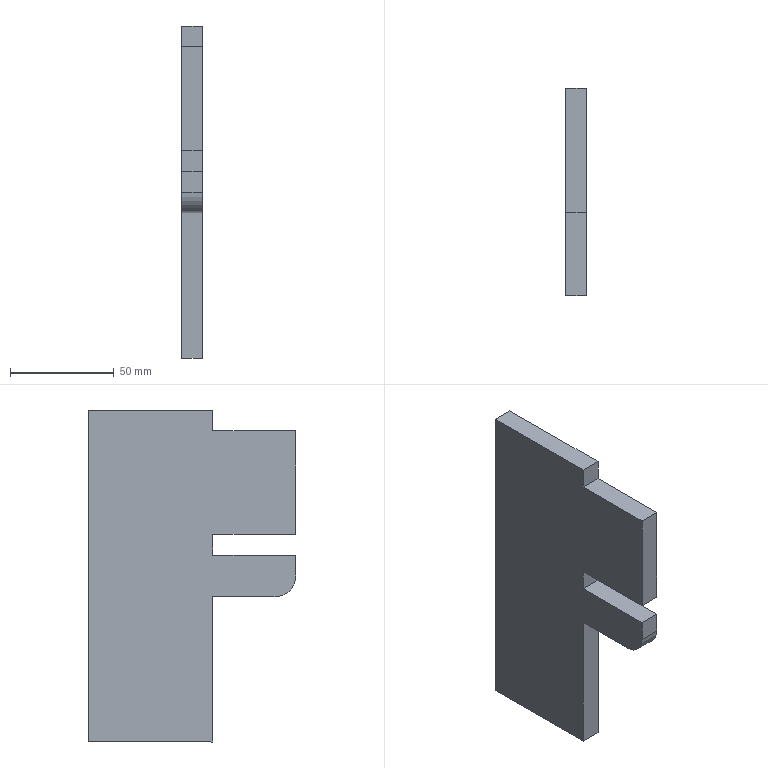Part | STEP file | cylinder mounting plate reinforcement--000.001--20240928 | 1 solid | 15 faces | box 10 x 100 x 160 mm | volume 123785 mm3 | plane 14 | cylinder 1 | commonest cylinder face diameters 20 x1
STEP:
#1=CARTESIAN_POINT('',(0.,0.,0.));
#2=DIRECTION('',(0.,0.,1.));
#3=DIRECTION('',(1.,0.,0.));
#4=AXIS2_PLACEMENT_3D('',#1,#2,#3);
#5=CARTESIAN_POINT('',(0.,-60.,90.));
#6=VERTEX_POINT('',#5);
#7=CARTESIAN_POINT('',(-10.,-60.,90.));
#8=VERTEX_POINT('',#7);
#9=CARTESIAN_POINT('',(657.,-60.,90.));
#10=DIRECTION('',(-1.,0.,0.));
#11=VECTOR('',#10,1.);
#12=LINE('',#9,#11);
#13=CARTESIAN_POINT('',(-221.5,-60.,-40.));
#14=DIRECTION('',(0.,-1.,0.));
#15=DIRECTION('',(-1.,0.,0.));
#16=AXIS2_PLACEMENT_3D('',#13,#14,#15);
#17=PLANE('',#16);
#18=CARTESIAN_POINT('',(-878.5,-130.));
#19=DIRECTION('',(1.,0.));
#20=VECTOR('',#19,1.);
#21=LINE('',#18,#20);
#22=(GEOMETRIC_REPRESENTATION_CONTEXT(2)PARAMETRIC_REPRESENTATION_CONTEXT()REPRESENTATION_CONTEXT('',''));
#23=DEFINITIONAL_REPRESENTATION('',(#21),#22);
#24=PCURVE('',#17,#23);
#25=CARTESIAN_POINT('',(657.,0.,90.));
#26=DIRECTION('',(0.,0.,1.));
#27=DIRECTION('',(0.,1.,0.));
#28=AXIS2_PLACEMENT_3D('',#25,#26,#27);
#29=PLANE('',#28);
#30=CARTESIAN_POINT('',(-60.,0.));
#31=DIRECTION('',(0.,1.));
#32=VECTOR('',#31,1.);
#33=LINE('',#30,#32);
#34=(GEOMETRIC_REPRESENTATION_CONTEXT(2)PARAMETRIC_REPRESENTATION_CONTEXT()REPRESENTATION_CONTEXT('',''));
#35=DEFINITIONAL_REPRESENTATION('',(#33),#34);
#36=PCURVE('',#29,#35);
#37=SURFACE_CURVE('',#12,(#24,#36),.PCURVE_S1.);
#38=EDGE_CURVE('',#6,#8,#37,.T.);
#39=ORIENTED_EDGE('',*,*,#38,.F.);
#40=CARTESIAN_POINT('',(0.,-60.,100.));
#41=VERTEX_POINT('',#40);
#42=CARTESIAN_POINT('',(0.,-60.,-40.));
#43=DIRECTION('',(0.,0.,1.));
#44=VECTOR('',#43,1.);
#45=LINE('',#42,#44);
#46=CARTESIAN_POINT('',(-221.5,0.));
#47=DIRECTION('',(0.,-1.));
#48=VECTOR('',#47,1.);
#49=LINE('',#46,#48);
#50=(GEOMETRIC_REPRESENTATION_CONTEXT(2)PARAMETRIC_REPRESENTATION_CONTEXT()REPRESENTATION_CONTEXT('',''));
#51=DEFINITIONAL_REPRESENTATION('',(#49),#50);
#52=PCURVE('',#17,#51);
#53=CARTESIAN_POINT('',(0.,-60.,1330.173));
#54=DIRECTION('',(-1.,0.,0.));
#55=DIRECTION('',(0.,-0.2756,-0.9613));
#56=AXIS2_PLACEMENT_3D('',#53,#54,#55);
#57=PLANE('',#56);
#58=CARTESIAN_POINT('',(1317.095,-377.671));
#59=DIRECTION('',(-0.9613,0.2756));
#60=VECTOR('',#59,1.);
#61=LINE('',#58,#60);
#62=(GEOMETRIC_REPRESENTATION_CONTEXT(2)PARAMETRIC_REPRESENTATION_CONTEXT()REPRESENTATION_CONTEXT('',''));
#63=DEFINITIONAL_REPRESENTATION('',(#61),#62);
#64=PCURVE('',#57,#63);
#65=SURFACE_CURVE('',#45,(#52,#64),.PCURVE_S1.);
#66=EDGE_CURVE('',#6,#41,#65,.T.);
#67=ORIENTED_EDGE('',*,*,#66,.T.);
#68=CARTESIAN_POINT('',(-10.,-60.,100.));
#69=VERTEX_POINT('',#68);
#70=CARTESIAN_POINT('',(657.,-60.,100.));
#71=DIRECTION('',(-1.,0.,0.));
#72=VECTOR('',#71,1.);
#73=LINE('',#70,#72);
#74=CARTESIAN_POINT('',(-878.5,-140.));
#75=DIRECTION('',(1.,0.));
#76=VECTOR('',#75,1.);
#77=LINE('',#74,#76);
#78=(GEOMETRIC_REPRESENTATION_CONTEXT(2)PARAMETRIC_REPRESENTATION_CONTEXT()REPRESENTATION_CONTEXT('',''));
#79=DEFINITIONAL_REPRESENTATION('',(#77),#78);
#80=PCURVE('',#17,#79);
#81=CARTESIAN_POINT('',(657.,0.,100.));
#82=DIRECTION('',(0.,0.,1.));
#83=DIRECTION('',(0.,1.,0.));
#84=AXIS2_PLACEMENT_3D('',#81,#82,#83);
#85=PLANE('',#84);
#86=CARTESIAN_POINT('',(-60.,0.));
#87=DIRECTION('',(0.,1.));
#88=VECTOR('',#87,1.);
#89=LINE('',#86,#88);
#90=(GEOMETRIC_REPRESENTATION_CONTEXT(2)PARAMETRIC_REPRESENTATION_CONTEXT()REPRESENTATION_CONTEXT('',''));
#91=DEFINITIONAL_REPRESENTATION('',(#89),#90);
#92=PCURVE('',#85,#91);
#93=SURFACE_CURVE('',#73,(#80,#92),.PCURVE_S1.);
#94=EDGE_CURVE('',#41,#69,#93,.T.);
#95=ORIENTED_EDGE('',*,*,#94,.T.);
#96=CARTESIAN_POINT('',(-10.,-60.,-40.));
#97=DIRECTION('',(0.,0.,1.));
#98=VECTOR('',#97,1.);
#99=LINE('',#96,#98);
#100=CARTESIAN_POINT('',(-211.5,0.));
#101=DIRECTION('',(0.,-1.));
#102=VECTOR('',#101,1.);
#103=LINE('',#100,#102);
#104=(GEOMETRIC_REPRESENTATION_CONTEXT(2)PARAMETRIC_REPRESENTATION_CONTEXT()REPRESENTATION_CONTEXT('',''));
#105=DEFINITIONAL_REPRESENTATION('',(#103),#104);
#106=PCURVE('',#17,#105);
#107=CARTESIAN_POINT('',(-10.,-60.,1330.173));
#108=DIRECTION('',(-1.,0.,0.));
#109=DIRECTION('',(0.,-0.2756,-0.9613));
#110=AXIS2_PLACEMENT_3D('',#107,#108,#109);
#111=PLANE('',#110);
#112=CARTESIAN_POINT('',(1317.095,-377.671));
#113=DIRECTION('',(-0.9613,0.2756));
#114=VECTOR('',#113,1.);
#115=LINE('',#112,#114);
#116=(GEOMETRIC_REPRESENTATION_CONTEXT(2)PARAMETRIC_REPRESENTATION_CONTEXT()REPRESENTATION_CONTEXT('',''));
#117=DEFINITIONAL_REPRESENTATION('',(#115),#116);
#118=PCURVE('',#111,#117);
#119=SURFACE_CURVE('',#99,(#106,#118),.PCURVE_S1.);
#120=EDGE_CURVE('',#8,#69,#119,.T.);
#121=ORIENTED_EDGE('',*,*,#120,.F.);
#122=EDGE_LOOP('',(#39,#67,#95,#121));
#123=FACE_BOUND('',#122,.T.);
#124=ADVANCED_FACE('',(#123),#17,.T.);
#125=CARTESIAN_POINT('',(-10.,-60.,70.));
#126=VERTEX_POINT('',#125);
#127=CARTESIAN_POINT('',(0.,-60.,70.));
#128=VERTEX_POINT('',#127);
#129=CARTESIAN_POINT('',(-221.5,-60.,70.));
#130=DIRECTION('',(1.,0.,0.));
#131=VECTOR('',#130,1.);
#132=LINE('',#129,#131);
#133=CARTESIAN_POINT('',(-221.5,-60.,-40.));
#134=DIRECTION('',(0.,-1.,0.));
#135=DIRECTION('',(-1.,0.,0.));
#136=AXIS2_PLACEMENT_3D('',#133,#134,#135);
#137=PLANE('',#136);
#138=CARTESIAN_POINT('',(0.,-110.));
#139=DIRECTION('',(-1.,0.));
#140=VECTOR('',#139,1.);
#141=LINE('',#138,#140);
#142=(GEOMETRIC_REPRESENTATION_CONTEXT(2)PARAMETRIC_REPRESENTATION_CONTEXT()REPRESENTATION_CONTEXT('',''));
#143=DEFINITIONAL_REPRESENTATION('',(#141),#142);
#144=PCURVE('',#137,#143);
#145=CARTESIAN_POINT('',(-110.,-60.,70.));
#146=DIRECTION('',(0.,0.,1.));
#147=DIRECTION('',(0.,-1.,0.));
#148=AXIS2_PLACEMENT_3D('',#145,#146,#147);
#149=PLANE('',#148);
#150=CARTESIAN_POINT('',(0.,-111.5));
#151=DIRECTION('',(0.,1.));
#152=VECTOR('',#151,1.);
#153=LINE('',#150,#152);
#154=(GEOMETRIC_REPRESENTATION_CONTEXT(2)PARAMETRIC_REPRESENTATION_CONTEXT()REPRESENTATION_CONTEXT('',''));
#155=DEFINITIONAL_REPRESENTATION('',(#153),#154);
#156=PCURVE('',#149,#155);
#157=SURFACE_CURVE('',#132,(#144,#156),.PCURVE_S1.);
#158=EDGE_CURVE('',#126,#128,#157,.T.);
#159=ORIENTED_EDGE('',*,*,#158,.F.);
#160=CARTESIAN_POINT('',(-10.,-60.,0.));
#161=VERTEX_POINT('',#160);
#162=CARTESIAN_POINT('',(-10.,-60.,-40.));
#163=DIRECTION('',(0.,0.,1.));
#164=VECTOR('',#163,1.);
#165=LINE('',#162,#164);
#166=CARTESIAN_POINT('',(-211.5,0.));
#167=DIRECTION('',(0.,-1.));
#168=VECTOR('',#167,1.);
#169=LINE('',#166,#168);
#170=(GEOMETRIC_REPRESENTATION_CONTEXT(2)PARAMETRIC_REPRESENTATION_CONTEXT()REPRESENTATION_CONTEXT('',''));
#171=DEFINITIONAL_REPRESENTATION('',(#169),#170);
#172=PCURVE('',#137,#171);
#173=CARTESIAN_POINT('',(1317.095,-377.671));
#174=DIRECTION('',(-0.9613,0.2756));
#175=VECTOR('',#174,1.);
#176=LINE('',#173,#175);
#177=(GEOMETRIC_REPRESENTATION_CONTEXT(2)PARAMETRIC_REPRESENTATION_CONTEXT()REPRESENTATION_CONTEXT('',''));
#178=DEFINITIONAL_REPRESENTATION('',(#176),#177);
#179=PCURVE('',#111,#178);
#180=SURFACE_CURVE('',#165,(#172,#179),.PCURVE_S1.);
#181=EDGE_CURVE('',#161,#126,#180,.T.);
#182=ORIENTED_EDGE('',*,*,#181,.F.);
#183=CARTESIAN_POINT('',(0.,-60.,0.));
#184=VERTEX_POINT('',#183);
#185=CARTESIAN_POINT('',(-110.,-60.,0.));
#186=DIRECTION('',(-1.,0.,0.));
#187=VECTOR('',#186,1.);
#188=LINE('',#185,#187);
#189=CARTESIAN_POINT('',(-111.5,-40.));
#190=DIRECTION('',(1.,0.));
#191=VECTOR('',#190,1.);
#192=LINE('',#189,#191);
#193=(GEOMETRIC_REPRESENTATION_CONTEXT(2)PARAMETRIC_REPRESENTATION_CONTEXT()REPRESENTATION_CONTEXT('',''));
#194=DEFINITIONAL_REPRESENTATION('',(#192),#193);
#195=PCURVE('',#137,#194);
#196=CARTESIAN_POINT('',(-110.,-60.,0.));
#197=DIRECTION('',(0.,0.,1.));
#198=DIRECTION('',(0.,-1.,0.));
#199=AXIS2_PLACEMENT_3D('',#196,#197,#198);
#200=PLANE('',#199);
#201=CARTESIAN_POINT('',(0.,0.));
#202=DIRECTION('',(0.,-1.));
#203=VECTOR('',#202,1.);
#204=LINE('',#201,#203);
#205=(GEOMETRIC_REPRESENTATION_CONTEXT(2)PARAMETRIC_REPRESENTATION_CONTEXT()REPRESENTATION_CONTEXT('',''));
#206=DEFINITIONAL_REPRESENTATION('',(#204),#205);
#207=PCURVE('',#200,#206);
#208=SURFACE_CURVE('',#188,(#195,#207),.PCURVE_S1.);
#209=EDGE_CURVE('',#184,#161,#208,.T.);
#210=ORIENTED_EDGE('',*,*,#209,.F.);
#211=CARTESIAN_POINT('',(0.,-60.,-40.));
#212=DIRECTION('',(0.,0.,1.));
#213=VECTOR('',#212,1.);
#214=LINE('',#211,#213);
#215=CARTESIAN_POINT('',(-221.5,0.));
#216=DIRECTION('',(0.,-1.));
#217=VECTOR('',#216,1.);
#218=LINE('',#215,#217);
#219=(GEOMETRIC_REPRESENTATION_CONTEXT(2)PARAMETRIC_REPRESENTATION_CONTEXT()REPRESENTATION_CONTEXT('',''));
#220=DEFINITIONAL_REPRESENTATION('',(#218),#219);
#221=PCURVE('',#137,#220);
#222=CARTESIAN_POINT('',(1317.095,-377.671));
#223=DIRECTION('',(-0.9613,0.2756));
#224=VECTOR('',#223,1.);
#225=LINE('',#222,#224);
#226=(GEOMETRIC_REPRESENTATION_CONTEXT(2)PARAMETRIC_REPRESENTATION_CONTEXT()REPRESENTATION_CONTEXT('',''));
#227=DEFINITIONAL_REPRESENTATION('',(#225),#226);
#228=PCURVE('',#57,#227);
#229=SURFACE_CURVE('',#214,(#221,#228),.PCURVE_S1.);
#230=EDGE_CURVE('',#184,#128,#229,.T.);
#231=ORIENTED_EDGE('',*,*,#230,.T.);
#232=EDGE_LOOP('',(#159,#182,#210,#231));
#233=FACE_BOUND('',#232,.T.);
#234=ADVANCED_FACE('',(#233),#137,.T.);
#235=CARTESIAN_POINT('',(0.,-60.,150.));
#236=VERTEX_POINT('',#235);
#237=CARTESIAN_POINT('',(-10.,-60.,150.));
#238=VERTEX_POINT('',#237);
#239=CARTESIAN_POINT('',(657.,-60.,150.));
#240=DIRECTION('',(-1.,0.,0.));
#241=VECTOR('',#240,1.);
#242=LINE('',#239,#241);
#243=CARTESIAN_POINT('',(-221.5,-60.,-40.));
#244=DIRECTION('',(0.,-1.,0.));
#245=DIRECTION('',(-1.,0.,0.));
#246=AXIS2_PLACEMENT_3D('',#243,#244,#245);
#247=PLANE('',#246);
#248=CARTESIAN_POINT('',(-878.5,-190.));
#249=DIRECTION('',(1.,0.));
#250=VECTOR('',#249,1.);
#251=LINE('',#248,#250);
#252=(GEOMETRIC_REPRESENTATION_CONTEXT(2)PARAMETRIC_REPRESENTATION_CONTEXT()REPRESENTATION_CONTEXT('',''));
#253=DEFINITIONAL_REPRESENTATION('',(#251),#252);
#254=PCURVE('',#247,#253);
#255=CARTESIAN_POINT('',(657.,0.,150.));
#256=DIRECTION('',(0.,0.,1.));
#257=DIRECTION('',(0.,1.,0.));
#258=AXIS2_PLACEMENT_3D('',#255,#256,#257);
#259=PLANE('',#258);
#260=CARTESIAN_POINT('',(-60.,0.));
#261=DIRECTION('',(0.,1.));
#262=VECTOR('',#261,1.);
#263=LINE('',#260,#262);
#264=(GEOMETRIC_REPRESENTATION_CONTEXT(2)PARAMETRIC_REPRESENTATION_CONTEXT()REPRESENTATION_CONTEXT('',''));
#265=DEFINITIONAL_REPRESENTATION('',(#263),#264);
#266=PCURVE('',#259,#265);
#267=SURFACE_CURVE('',#242,(#254,#266),.PCURVE_S1.);
#268=EDGE_CURVE('',#236,#238,#267,.T.);
#269=ORIENTED_EDGE('',*,*,#268,.F.);
#270=CARTESIAN_POINT('',(0.,-60.,160.));
#271=VERTEX_POINT('',#270);
#272=CARTESIAN_POINT('',(0.,-60.,-40.));
#273=DIRECTION('',(0.,0.,1.));
#274=VECTOR('',#273,1.);
#275=LINE('',#272,#274);
#276=CARTESIAN_POINT('',(-221.5,0.));
#277=DIRECTION('',(0.,-1.));
#278=VECTOR('',#277,1.);
#279=LINE('',#276,#278);
#280=(GEOMETRIC_REPRESENTATION_CONTEXT(2)PARAMETRIC_REPRESENTATION_CONTEXT()REPRESENTATION_CONTEXT('',''));
#281=DEFINITIONAL_REPRESENTATION('',(#279),#280);
#282=PCURVE('',#247,#281);
#283=CARTESIAN_POINT('',(1317.095,-377.671));
#284=DIRECTION('',(-0.9613,0.2756));
#285=VECTOR('',#284,1.);
#286=LINE('',#283,#285);
#287=(GEOMETRIC_REPRESENTATION_CONTEXT(2)PARAMETRIC_REPRESENTATION_CONTEXT()REPRESENTATION_CONTEXT('',''));
#288=DEFINITIONAL_REPRESENTATION('',(#286),#287);
#289=PCURVE('',#57,#288);
#290=SURFACE_CURVE('',#275,(#282,#289),.PCURVE_S1.);
#291=EDGE_CURVE('',#236,#271,#290,.T.);
#292=ORIENTED_EDGE('',*,*,#291,.T.);
#293=CARTESIAN_POINT('',(-10.,-60.,160.));
#294=VERTEX_POINT('',#293);
#295=CARTESIAN_POINT('',(2.5,-60.,160.));
#296=DIRECTION('',(1.,0.,0.));
#297=VECTOR('',#296,1.);
#298=LINE('',#295,#297);
#299=CARTESIAN_POINT('',(-224.,-200.));
#300=DIRECTION('',(-1.,0.));
#301=VECTOR('',#300,1.);
#302=LINE('',#299,#301);
#303=(GEOMETRIC_REPRESENTATION_CONTEXT(2)PARAMETRIC_REPRESENTATION_CONTEXT()REPRESENTATION_CONTEXT('',''));
#304=DEFINITIONAL_REPRESENTATION('',(#302),#303);
#305=PCURVE('',#247,#304);
#306=CARTESIAN_POINT('',(2.5,-90.,160.));
#307=DIRECTION('',(0.,0.,1.));
#308=DIRECTION('',(0.,1.,0.));
#309=AXIS2_PLACEMENT_3D('',#306,#307,#308);
#310=PLANE('',#309);
#311=CARTESIAN_POINT('',(30.,0.));
#312=DIRECTION('',(0.,-1.));
#313=VECTOR('',#312,1.);
#314=LINE('',#311,#313);
#315=(GEOMETRIC_REPRESENTATION_CONTEXT(2)PARAMETRIC_REPRESENTATION_CONTEXT()REPRESENTATION_CONTEXT('',''));
#316=DEFINITIONAL_REPRESENTATION('',(#314),#315);
#317=PCURVE('',#310,#316);
#318=SURFACE_CURVE('',#298,(#305,#317),.PCURVE_S1.);
#319=EDGE_CURVE('',#294,#271,#318,.T.);
#320=ORIENTED_EDGE('',*,*,#319,.F.);
#321=CARTESIAN_POINT('',(-10.,-60.,-40.));
#322=DIRECTION('',(0.,0.,1.));
#323=VECTOR('',#322,1.);
#324=LINE('',#321,#323);
#325=CARTESIAN_POINT('',(-211.5,0.));
#326=DIRECTION('',(0.,-1.));
#327=VECTOR('',#326,1.);
#328=LINE('',#325,#327);
#329=(GEOMETRIC_REPRESENTATION_CONTEXT(2)PARAMETRIC_REPRESENTATION_CONTEXT()REPRESENTATION_CONTEXT('',''));
#330=DEFINITIONAL_REPRESENTATION('',(#328),#329);
#331=PCURVE('',#247,#330);
#332=CARTESIAN_POINT('',(1317.095,-377.671));
#333=DIRECTION('',(-0.9613,0.2756));
#334=VECTOR('',#333,1.);
#335=LINE('',#332,#334);
#336=(GEOMETRIC_REPRESENTATION_CONTEXT(2)PARAMETRIC_REPRESENTATION_CONTEXT()REPRESENTATION_CONTEXT('',''));
#337=DEFINITIONAL_REPRESENTATION('',(#335),#336);
#338=PCURVE('',#111,#337);
#339=SURFACE_CURVE('',#324,(#331,#338),.PCURVE_S1.);
#340=EDGE_CURVE('',#238,#294,#339,.T.);
#341=ORIENTED_EDGE('',*,*,#340,.F.);
#342=EDGE_LOOP('',(#269,#292,#320,#341));
#343=FACE_BOUND('',#342,.T.);
#344=ADVANCED_FACE('',(#343),#247,.T.);
#345=CARTESIAN_POINT('',(-10.,-90.,70.));
#346=VERTEX_POINT('',#345);
#347=CARTESIAN_POINT('',(-10.,-60.,70.));
#348=DIRECTION('',(0.,-1.,0.));
#349=VECTOR('',#348,1.);
#350=LINE('',#347,#349);
#351=CARTESIAN_POINT('',(1211.356,-347.351));
#352=DIRECTION('',(0.2756,0.9613));
#353=VECTOR('',#352,1.);
#354=LINE('',#351,#353);
#355=(GEOMETRIC_REPRESENTATION_CONTEXT(2)PARAMETRIC_REPRESENTATION_CONTEXT()REPRESENTATION_CONTEXT('',''));
#356=DEFINITIONAL_REPRESENTATION('',(#354),#355);
#357=PCURVE('',#111,#356);
#358=CARTESIAN_POINT('',(0.,100.));
#359=DIRECTION('',(1.,0.));
#360=VECTOR('',#359,1.);
#361=LINE('',#358,#360);
#362=(GEOMETRIC_REPRESENTATION_CONTEXT(2)PARAMETRIC_REPRESENTATION_CONTEXT()REPRESENTATION_CONTEXT('',''));
#363=DEFINITIONAL_REPRESENTATION('',(#361),#362);
#364=PCURVE('',#149,#363);
#365=SURFACE_CURVE('',#350,(#357,#364),.PCURVE_S1.);
#366=EDGE_CURVE('',#126,#346,#365,.T.);
#367=ORIENTED_EDGE('',*,*,#366,.T.);
#368=CARTESIAN_POINT('',(-10.,-100.,80.));
#369=VERTEX_POINT('',#368);
#370=CARTESIAN_POINT('',(-10.,-90.,80.));
#371=DIRECTION('',(-1.,0.,0.));
#372=DIRECTION('',(0.,-1.,0.));
#373=AXIS2_PLACEMENT_3D('',#370,#371,#372);
#374=CIRCLE('',#373,10.);
#375=CARTESIAN_POINT('',(1210.013,-315.757));
#376=DIRECTION('',(0.2756,0.9613));
#377=AXIS2_PLACEMENT_2D('',#375,#376);
#378=CIRCLE('',#377,10.);
#379=(GEOMETRIC_REPRESENTATION_CONTEXT(2)PARAMETRIC_REPRESENTATION_CONTEXT()REPRESENTATION_CONTEXT('',''));
#380=DEFINITIONAL_REPRESENTATION('',(#378),#379);
#381=PCURVE('',#111,#380);
#382=CARTESIAN_POINT('',(-110.,-90.,80.));
#383=DIRECTION('',(1.,0.,0.));
#384=DIRECTION('',(0.,-1.,0.));
#385=AXIS2_PLACEMENT_3D('',#382,#383,#384);
#386=CYLINDRICAL_SURFACE('',#385,10.);
#387=CARTESIAN_POINT('',(6.283,100.));
#388=DIRECTION('',(-1.,0.));
#389=VECTOR('',#388,1.);
#390=LINE('',#387,#389);
#391=(GEOMETRIC_REPRESENTATION_CONTEXT(2)PARAMETRIC_REPRESENTATION_CONTEXT()REPRESENTATION_CONTEXT('',''));
#392=DEFINITIONAL_REPRESENTATION('',(#390),#391);
#393=PCURVE('',#386,#392);
#394=SURFACE_CURVE('',#374,(#381,#393),.PCURVE_S1.);
#395=EDGE_CURVE('',#346,#369,#394,.T.);
#396=ORIENTED_EDGE('',*,*,#395,.T.);
#397=CARTESIAN_POINT('',(-10.,-100.,90.));
#398=VERTEX_POINT('',#397);
#399=CARTESIAN_POINT('',(-10.,-100.,-40.));
#400=DIRECTION('',(0.,0.,1.));
#401=VECTOR('',#400,1.);
#402=LINE('',#399,#401);
#403=CARTESIAN_POINT('',(1328.121,-339.22));
#404=DIRECTION('',(-0.9613,0.2756));
#405=VECTOR('',#404,1.);
#406=LINE('',#403,#405);
#407=(GEOMETRIC_REPRESENTATION_CONTEXT(2)PARAMETRIC_REPRESENTATION_CONTEXT()REPRESENTATION_CONTEXT('',''));
#408=DEFINITIONAL_REPRESENTATION('',(#406),#407);
#409=PCURVE('',#111,#408);
#410=CARTESIAN_POINT('',(-221.5,-100.,-40.));
#411=DIRECTION('',(0.,-1.,0.));
#412=DIRECTION('',(-1.,0.,0.));
#413=AXIS2_PLACEMENT_3D('',#410,#411,#412);
#414=PLANE('',#413);
#415=CARTESIAN_POINT('',(-211.5,0.));
#416=DIRECTION('',(0.,-1.));
#417=VECTOR('',#416,1.);
#418=LINE('',#415,#417);
#419=(GEOMETRIC_REPRESENTATION_CONTEXT(2)PARAMETRIC_REPRESENTATION_CONTEXT()REPRESENTATION_CONTEXT('',''));
#420=DEFINITIONAL_REPRESENTATION('',(#418),#419);
#421=PCURVE('',#414,#420);
#422=SURFACE_CURVE('',#402,(#409,#421),.PCURVE_S1.);
#423=EDGE_CURVE('',#369,#398,#422,.T.);
#424=ORIENTED_EDGE('',*,*,#423,.T.);
#425=CARTESIAN_POINT('',(-10.,-60.,90.));
#426=DIRECTION('',(0.,1.,0.));
#427=VECTOR('',#426,1.);
#428=LINE('',#425,#427);
#429=CARTESIAN_POINT('',(1192.131,-341.838));
#430=DIRECTION('',(-0.2756,-0.9613));
#431=VECTOR('',#430,1.);
#432=LINE('',#429,#431);
#433=(GEOMETRIC_REPRESENTATION_CONTEXT(2)PARAMETRIC_REPRESENTATION_CONTEXT()REPRESENTATION_CONTEXT('',''));
#434=DEFINITIONAL_REPRESENTATION('',(#432),#433);
#435=PCURVE('',#111,#434);
#436=CARTESIAN_POINT('',(-60.,667.));
#437=DIRECTION('',(1.,0.));
#438=VECTOR('',#437,1.);
#439=LINE('',#436,#438);
#440=(GEOMETRIC_REPRESENTATION_CONTEXT(2)PARAMETRIC_REPRESENTATION_CONTEXT()REPRESENTATION_CONTEXT('',''));
#441=DEFINITIONAL_REPRESENTATION('',(#439),#440);
#442=PCURVE('',#29,#441);
#443=SURFACE_CURVE('',#428,(#435,#442),.PCURVE_S1.);
#444=EDGE_CURVE('',#398,#8,#443,.T.);
#445=ORIENTED_EDGE('',*,*,#444,.T.);
#446=ORIENTED_EDGE('',*,*,#120,.T.);
#447=CARTESIAN_POINT('',(-10.,-100.,100.));
#448=VERTEX_POINT('',#447);
#449=CARTESIAN_POINT('',(-10.,-60.,100.));
#450=DIRECTION('',(0.,1.,0.));
#451=VECTOR('',#450,1.);
#452=LINE('',#449,#451);
#453=CARTESIAN_POINT('',(1182.518,-339.082));
#454=DIRECTION('',(-0.2756,-0.9613));
#455=VECTOR('',#454,1.);
#456=LINE('',#453,#455);
#457=(GEOMETRIC_REPRESENTATION_CONTEXT(2)PARAMETRIC_REPRESENTATION_CONTEXT()REPRESENTATION_CONTEXT('',''));
#458=DEFINITIONAL_REPRESENTATION('',(#456),#457);
#459=PCURVE('',#111,#458);
#460=CARTESIAN_POINT('',(-60.,667.));
#461=DIRECTION('',(1.,0.));
#462=VECTOR('',#461,1.);
#463=LINE('',#460,#462);
#464=(GEOMETRIC_REPRESENTATION_CONTEXT(2)PARAMETRIC_REPRESENTATION_CONTEXT()REPRESENTATION_CONTEXT('',''));
#465=DEFINITIONAL_REPRESENTATION('',(#463),#464);
#466=PCURVE('',#85,#465);
#467=SURFACE_CURVE('',#452,(#459,#466),.PCURVE_S1.);
#468=EDGE_CURVE('',#448,#69,#467,.T.);
#469=ORIENTED_EDGE('',*,*,#468,.F.);
#470=CARTESIAN_POINT('',(-10.,-100.,150.));
#471=VERTEX_POINT('',#470);
#472=CARTESIAN_POINT('',(-10.,-100.,-40.));
#473=DIRECTION('',(0.,0.,1.));
#474=VECTOR('',#473,1.);
#475=LINE('',#472,#474);
#476=CARTESIAN_POINT('',(1328.121,-339.22));
#477=DIRECTION('',(-0.9613,0.2756));
#478=VECTOR('',#477,1.);
#479=LINE('',#476,#478);
#480=(GEOMETRIC_REPRESENTATION_CONTEXT(2)PARAMETRIC_REPRESENTATION_CONTEXT()REPRESENTATION_CONTEXT('',''));
#481=DEFINITIONAL_REPRESENTATION('',(#479),#480);
#482=PCURVE('',#111,#481);
#483=CARTESIAN_POINT('',(-221.5,-100.,-40.));
#484=DIRECTION('',(0.,-1.,0.));
#485=DIRECTION('',(-1.,0.,0.));
#486=AXIS2_PLACEMENT_3D('',#483,#484,#485);
#487=PLANE('',#486);
#488=CARTESIAN_POINT('',(-211.5,0.));
#489=DIRECTION('',(0.,-1.));
#490=VECTOR('',#489,1.);
#491=LINE('',#488,#490);
#492=(GEOMETRIC_REPRESENTATION_CONTEXT(2)PARAMETRIC_REPRESENTATION_CONTEXT()REPRESENTATION_CONTEXT('',''));
#493=DEFINITIONAL_REPRESENTATION('',(#491),#492);
#494=PCURVE('',#487,#493);
#495=SURFACE_CURVE('',#475,(#482,#494),.PCURVE_S1.);
#496=EDGE_CURVE('',#448,#471,#495,.T.);
#497=ORIENTED_EDGE('',*,*,#496,.T.);
#498=CARTESIAN_POINT('',(-10.,-60.,150.));
#499=DIRECTION('',(0.,1.,0.));
#500=VECTOR('',#499,1.);
#501=LINE('',#498,#500);
#502=CARTESIAN_POINT('',(1134.455,-325.3));
#503=DIRECTION('',(-0.2756,-0.9613));
#504=VECTOR('',#503,1.);
#505=LINE('',#502,#504);
#506=(GEOMETRIC_REPRESENTATION_CONTEXT(2)PARAMETRIC_REPRESENTATION_CONTEXT()REPRESENTATION_CONTEXT('',''));
#507=DEFINITIONAL_REPRESENTATION('',(#505),#506);
#508=PCURVE('',#111,#507);
#509=CARTESIAN_POINT('',(-60.,667.));
#510=DIRECTION('',(1.,0.));
#511=VECTOR('',#510,1.);
#512=LINE('',#509,#511);
#513=(GEOMETRIC_REPRESENTATION_CONTEXT(2)PARAMETRIC_REPRESENTATION_CONTEXT()REPRESENTATION_CONTEXT('',''));
#514=DEFINITIONAL_REPRESENTATION('',(#512),#513);
#515=PCURVE('',#259,#514);
#516=SURFACE_CURVE('',#501,(#508,#515),.PCURVE_S1.);
#517=EDGE_CURVE('',#471,#238,#516,.T.);
#518=ORIENTED_EDGE('',*,*,#517,.T.);
#519=ORIENTED_EDGE('',*,*,#340,.T.);
#520=CARTESIAN_POINT('',(-10.,0.,160.));
#521=VERTEX_POINT('',#520);
#522=CARTESIAN_POINT('',(-10.,-60.,160.));
#523=DIRECTION('',(0.,1.,0.));
#524=VECTOR('',#523,1.);
#525=LINE('',#522,#524);
#526=CARTESIAN_POINT('',(1124.843,-322.543));
#527=DIRECTION('',(-0.2756,-0.9613));
#528=VECTOR('',#527,1.);
#529=LINE('',#526,#528);
#530=(GEOMETRIC_REPRESENTATION_CONTEXT(2)PARAMETRIC_REPRESENTATION_CONTEXT()REPRESENTATION_CONTEXT('',''));
#531=DEFINITIONAL_REPRESENTATION('',(#529),#530);
#532=PCURVE('',#111,#531);
#533=CARTESIAN_POINT('',(30.,12.5));
#534=DIRECTION('',(1.,0.));
#535=VECTOR('',#534,1.);
#536=LINE('',#533,#535);
#537=(GEOMETRIC_REPRESENTATION_CONTEXT(2)PARAMETRIC_REPRESENTATION_CONTEXT()REPRESENTATION_CONTEXT('',''));
#538=DEFINITIONAL_REPRESENTATION('',(#536),#537);
#539=PCURVE('',#310,#538);
#540=SURFACE_CURVE('',#525,(#532,#539),.PCURVE_S1.);
#541=EDGE_CURVE('',#294,#521,#540,.T.);
#542=ORIENTED_EDGE('',*,*,#541,.T.);
#543=CARTESIAN_POINT('',(-10.,0.,0.));
#544=VERTEX_POINT('',#543);
#545=CARTESIAN_POINT('',(-10.,0.,1950.173));
#546=DIRECTION('',(0.,0.,-1.));
#547=VECTOR('',#546,1.);
#548=LINE('',#545,#547);
#549=CARTESIAN_POINT('',(-612.52,113.219));
#550=DIRECTION('',(0.9613,-0.2756));
#551=VECTOR('',#550,1.);
#552=LINE('',#549,#551);
#553=(GEOMETRIC_REPRESENTATION_CONTEXT(2)PARAMETRIC_REPRESENTATION_CONTEXT()REPRESENTATION_CONTEXT('',''));
#554=DEFINITIONAL_REPRESENTATION('',(#552),#553);
#555=PCURVE('',#111,#554);
#556=CARTESIAN_POINT('',(-110.,0.,1950.173));
#557=DIRECTION('',(0.,-1.,0.));
#558=DIRECTION('',(0.,0.,1.));
#559=AXIS2_PLACEMENT_3D('',#556,#557,#558);
#560=PLANE('',#559);
#561=CARTESIAN_POINT('',(0.,-100.));
#562=DIRECTION('',(-1.,0.));
#563=VECTOR('',#562,1.);
#564=LINE('',#561,#563);
#565=(GEOMETRIC_REPRESENTATION_CONTEXT(2)PARAMETRIC_REPRESENTATION_CONTEXT()REPRESENTATION_CONTEXT('',''));
#566=DEFINITIONAL_REPRESENTATION('',(#564),#565);
#567=PCURVE('',#560,#566);
#568=SURFACE_CURVE('',#548,(#555,#567),.PCURVE_S1.);
#569=EDGE_CURVE('',#521,#544,#568,.T.);
#570=ORIENTED_EDGE('',*,*,#569,.T.);
#571=CARTESIAN_POINT('',(-10.,-60.,0.));
#572=DIRECTION('',(0.,1.,0.));
#573=VECTOR('',#572,1.);
#574=LINE('',#571,#573);
#575=CARTESIAN_POINT('',(1278.645,-366.645));
#576=DIRECTION('',(-0.2756,-0.9613));
#577=VECTOR('',#576,1.);
#578=LINE('',#575,#577);
#579=(GEOMETRIC_REPRESENTATION_CONTEXT(2)PARAMETRIC_REPRESENTATION_CONTEXT()REPRESENTATION_CONTEXT('',''));
#580=DEFINITIONAL_REPRESENTATION('',(#578),#579);
#581=PCURVE('',#111,#580);
#582=CARTESIAN_POINT('',(0.,100.));
#583=DIRECTION('',(-1.,0.));
#584=VECTOR('',#583,1.);
#585=LINE('',#582,#584);
#586=(GEOMETRIC_REPRESENTATION_CONTEXT(2)PARAMETRIC_REPRESENTATION_CONTEXT()REPRESENTATION_CONTEXT('',''));
#587=DEFINITIONAL_REPRESENTATION('',(#585),#586);
#588=PCURVE('',#200,#587);
#589=SURFACE_CURVE('',#574,(#581,#588),.PCURVE_S1.);
#590=EDGE_CURVE('',#161,#544,#589,.T.);
#591=ORIENTED_EDGE('',*,*,#590,.F.);
#592=ORIENTED_EDGE('',*,*,#181,.T.);
#593=EDGE_LOOP('',(#367,#396,#424,#445,#446,#469,#497,#518,#519,#542,#570,#591,#592));
#594=FACE_BOUND('',#593,.T.);
#595=ADVANCED_FACE('',(#594),#111,.T.);
#596=CARTESIAN_POINT('',(0.,-100.,80.));
#597=VERTEX_POINT('',#596);
#598=CARTESIAN_POINT('',(0.,-100.,90.));
#599=VERTEX_POINT('',#598);
#600=CARTESIAN_POINT('',(0.,-100.,-40.));
#601=DIRECTION('',(0.,0.,1.));
#602=VECTOR('',#601,1.);
#603=LINE('',#600,#602);
#604=CARTESIAN_POINT('',(1328.121,-339.22));
#605=DIRECTION('',(-0.9613,0.2756));
#606=VECTOR('',#605,1.);
#607=LINE('',#604,#606);
#608=(GEOMETRIC_REPRESENTATION_CONTEXT(2)PARAMETRIC_REPRESENTATION_CONTEXT()REPRESENTATION_CONTEXT('',''));
#609=DEFINITIONAL_REPRESENTATION('',(#607),#608);
#610=PCURVE('',#57,#609);
#611=CARTESIAN_POINT('',(-221.5,0.));
#612=DIRECTION('',(0.,-1.));
#613=VECTOR('',#612,1.);
#614=LINE('',#611,#613);
#615=(GEOMETRIC_REPRESENTATION_CONTEXT(2)PARAMETRIC_REPRESENTATION_CONTEXT()REPRESENTATION_CONTEXT('',''));
#616=DEFINITIONAL_REPRESENTATION('',(#614),#615);
#617=PCURVE('',#414,#616);
#618=SURFACE_CURVE('',#603,(#610,#617),.PCURVE_S1.);
#619=EDGE_CURVE('',#597,#599,#618,.T.);
#620=ORIENTED_EDGE('',*,*,#619,.F.);
#621=CARTESIAN_POINT('',(0.,-90.,70.));
#622=VERTEX_POINT('',#621);
#623=CARTESIAN_POINT('',(0.,-90.,80.));
#624=DIRECTION('',(1.,0.,0.));
#625=DIRECTION('',(0.,-1.,0.));
#626=AXIS2_PLACEMENT_3D('',#623,#624,#625);
#627=CIRCLE('',#626,10.);
#628=CARTESIAN_POINT('',(1212.769,-306.144));
#629=CARTESIAN_POINT('',(1229.419,-310.918));
#630=CARTESIAN_POINT('',(1216.959,-322.95));
#631=CARTESIAN_POINT('',(1204.5,-334.982));
#632=CARTESIAN_POINT('',(1200.31,-318.176));
#633=CARTESIAN_POINT('',(1196.12,-301.37));
#634=CARTESIAN_POINT('',(1212.769,-306.144));
#635=(BOUNDED_CURVE()B_SPLINE_CURVE(2,(#628,#629,#630,#631,#632,#633,#634),.UNSPECIFIED.,.T.,.F.)B_SPLINE_CURVE_WITH_KNOTS((1,2,2,2,2,1),(-2.094,0.,2.094,4.189,6.283,8.378),.UNSPECIFIED.)CURVE()GEOMETRIC_REPRESENTATION_ITEM()RATIONAL_B_SPLINE_CURVE((1.,0.5,1.,0.5,1.,0.5,1.))REPRESENTATION_ITEM(''));
#636=(GEOMETRIC_REPRESENTATION_CONTEXT(2)PARAMETRIC_REPRESENTATION_CONTEXT()REPRESENTATION_CONTEXT('',''));
#637=DEFINITIONAL_REPRESENTATION('',(#635),#636);
#638=PCURVE('',#57,#637);
#639=CARTESIAN_POINT('',(0.,110.));
#640=DIRECTION('',(1.,0.));
#641=VECTOR('',#640,1.);
#642=LINE('',#639,#641);
#643=(GEOMETRIC_REPRESENTATION_CONTEXT(2)PARAMETRIC_REPRESENTATION_CONTEXT()REPRESENTATION_CONTEXT('',''));
#644=DEFINITIONAL_REPRESENTATION('',(#642),#643);
#645=PCURVE('',#386,#644);
#646=SURFACE_CURVE('',#627,(#638,#645),.PCURVE_S1.);
#647=EDGE_CURVE('',#597,#622,#646,.T.);
#648=ORIENTED_EDGE('',*,*,#647,.T.);
#649=CARTESIAN_POINT('',(0.,-60.,70.));
#650=DIRECTION('',(0.,1.,0.));
#651=VECTOR('',#650,1.);
#652=LINE('',#649,#651);
#653=CARTESIAN_POINT('',(1211.356,-347.351));
#654=DIRECTION('',(-0.2756,-0.9613));
#655=VECTOR('',#654,1.);
#656=LINE('',#653,#655);
#657=(GEOMETRIC_REPRESENTATION_CONTEXT(2)PARAMETRIC_REPRESENTATION_CONTEXT()REPRESENTATION_CONTEXT('',''));
#658=DEFINITIONAL_REPRESENTATION('',(#656),#657);
#659=PCURVE('',#57,#658);
#660=CARTESIAN_POINT('',(0.,110.));
#661=DIRECTION('',(-1.,0.));
#662=VECTOR('',#661,1.);
#663=LINE('',#660,#662);
#664=(GEOMETRIC_REPRESENTATION_CONTEXT(2)PARAMETRIC_REPRESENTATION_CONTEXT()REPRESENTATION_CONTEXT('',''));
#665=DEFINITIONAL_REPRESENTATION('',(#663),#664);
#666=PCURVE('',#149,#665);
#667=SURFACE_CURVE('',#652,(#659,#666),.PCURVE_S1.);
#668=EDGE_CURVE('',#622,#128,#667,.T.);
#669=ORIENTED_EDGE('',*,*,#668,.T.);
#670=ORIENTED_EDGE('',*,*,#230,.F.);
#671=CARTESIAN_POINT('',(0.,0.,0.));
#672=VERTEX_POINT('',#671);
#673=CARTESIAN_POINT('',(0.,-60.,0.));
#674=DIRECTION('',(0.,1.,0.));
#675=VECTOR('',#674,1.);
#676=LINE('',#673,#675);
#677=CARTESIAN_POINT('',(1278.645,-366.645));
#678=DIRECTION('',(-0.2756,-0.9613));
#679=VECTOR('',#678,1.);
#680=LINE('',#677,#679);
#681=(GEOMETRIC_REPRESENTATION_CONTEXT(2)PARAMETRIC_REPRESENTATION_CONTEXT()REPRESENTATION_CONTEXT('',''));
#682=DEFINITIONAL_REPRESENTATION('',(#680),#681);
#683=PCURVE('',#57,#682);
#684=CARTESIAN_POINT('',(0.,110.));
#685=DIRECTION('',(-1.,0.));
#686=VECTOR('',#685,1.);
#687=LINE('',#684,#686);
#688=(GEOMETRIC_REPRESENTATION_CONTEXT(2)PARAMETRIC_REPRESENTATION_CONTEXT()REPRESENTATION_CONTEXT('',''));
#689=DEFINITIONAL_REPRESENTATION('',(#687),#688);
#690=PCURVE('',#200,#689);
#691=SURFACE_CURVE('',#676,(#683,#690),.PCURVE_S1.);
#692=EDGE_CURVE('',#184,#672,#691,.T.);
#693=ORIENTED_EDGE('',*,*,#692,.T.);
#694=CARTESIAN_POINT('',(0.,0.,160.));
#695=VERTEX_POINT('',#694);
#696=CARTESIAN_POINT('',(0.,0.,1950.173));
#697=DIRECTION('',(0.,0.,-1.));
#698=VECTOR('',#697,1.);
#699=LINE('',#696,#698);
#700=CARTESIAN_POINT('',(-612.52,113.219));
#701=DIRECTION('',(0.9613,-0.2756));
#702=VECTOR('',#701,1.);
#703=LINE('',#700,#702);
#704=(GEOMETRIC_REPRESENTATION_CONTEXT(2)PARAMETRIC_REPRESENTATION_CONTEXT()REPRESENTATION_CONTEXT('',''));
#705=DEFINITIONAL_REPRESENTATION('',(#703),#704);
#706=PCURVE('',#57,#705);
#707=CARTESIAN_POINT('',(0.,-110.));
#708=DIRECTION('',(-1.,0.));
#709=VECTOR('',#708,1.);
#710=LINE('',#707,#709);
#711=(GEOMETRIC_REPRESENTATION_CONTEXT(2)PARAMETRIC_REPRESENTATION_CONTEXT()REPRESENTATION_CONTEXT('',''));
#712=DEFINITIONAL_REPRESENTATION('',(#710),#711);
#713=PCURVE('',#560,#712);
#714=SURFACE_CURVE('',#699,(#706,#713),.PCURVE_S1.);
#715=EDGE_CURVE('',#695,#672,#714,.T.);
#716=ORIENTED_EDGE('',*,*,#715,.F.);
#717=CARTESIAN_POINT('',(0.,-60.,160.));
#718=DIRECTION('',(0.,1.,0.));
#719=VECTOR('',#718,1.);
#720=LINE('',#717,#719);
#721=CARTESIAN_POINT('',(1124.843,-322.543));
#722=DIRECTION('',(-0.2756,-0.9613));
#723=VECTOR('',#722,1.);
#724=LINE('',#721,#723);
#725=(GEOMETRIC_REPRESENTATION_CONTEXT(2)PARAMETRIC_REPRESENTATION_CONTEXT()REPRESENTATION_CONTEXT('',''));
#726=DEFINITIONAL_REPRESENTATION('',(#724),#725);
#727=PCURVE('',#57,#726);
#728=CARTESIAN_POINT('',(30.,2.5));
#729=DIRECTION('',(1.,0.));
#730=VECTOR('',#729,1.);
#731=LINE('',#728,#730);
#732=(GEOMETRIC_REPRESENTATION_CONTEXT(2)PARAMETRIC_REPRESENTATION_CONTEXT()REPRESENTATION_CONTEXT('',''));
#733=DEFINITIONAL_REPRESENTATION('',(#731),#732);
#734=PCURVE('',#310,#733);
#735=SURFACE_CURVE('',#720,(#727,#734),.PCURVE_S1.);
#736=EDGE_CURVE('',#271,#695,#735,.T.);
#737=ORIENTED_EDGE('',*,*,#736,.F.);
#738=ORIENTED_EDGE('',*,*,#291,.F.);
#739=CARTESIAN_POINT('',(0.,-100.,150.));
#740=VERTEX_POINT('',#739);
#741=CARTESIAN_POINT('',(0.,-60.,150.));
#742=DIRECTION('',(0.,1.,0.));
#743=VECTOR('',#742,1.);
#744=LINE('',#741,#743);
#745=CARTESIAN_POINT('',(1134.455,-325.3));
#746=DIRECTION('',(-0.2756,-0.9613));
#747=VECTOR('',#746,1.);
#748=LINE('',#745,#747);
#749=(GEOMETRIC_REPRESENTATION_CONTEXT(2)PARAMETRIC_REPRESENTATION_CONTEXT()REPRESENTATION_CONTEXT('',''));
#750=DEFINITIONAL_REPRESENTATION('',(#748),#749);
#751=PCURVE('',#57,#750);
#752=CARTESIAN_POINT('',(-60.,657.));
#753=DIRECTION('',(1.,0.));
#754=VECTOR('',#753,1.);
#755=LINE('',#752,#754);
#756=(GEOMETRIC_REPRESENTATION_CONTEXT(2)PARAMETRIC_REPRESENTATION_CONTEXT()REPRESENTATION_CONTEXT('',''));
#757=DEFINITIONAL_REPRESENTATION('',(#755),#756);
#758=PCURVE('',#259,#757);
#759=SURFACE_CURVE('',#744,(#751,#758),.PCURVE_S1.);
#760=EDGE_CURVE('',#740,#236,#759,.T.);
#761=ORIENTED_EDGE('',*,*,#760,.F.);
#762=CARTESIAN_POINT('',(0.,-100.,100.));
#763=VERTEX_POINT('',#762);
#764=CARTESIAN_POINT('',(0.,-100.,-40.));
#765=DIRECTION('',(0.,0.,1.));
#766=VECTOR('',#765,1.);
#767=LINE('',#764,#766);
#768=CARTESIAN_POINT('',(1328.121,-339.22));
#769=DIRECTION('',(-0.9613,0.2756));
#770=VECTOR('',#769,1.);
#771=LINE('',#768,#770);
#772=(GEOMETRIC_REPRESENTATION_CONTEXT(2)PARAMETRIC_REPRESENTATION_CONTEXT()REPRESENTATION_CONTEXT('',''));
#773=DEFINITIONAL_REPRESENTATION('',(#771),#772);
#774=PCURVE('',#57,#773);
#775=CARTESIAN_POINT('',(-221.5,0.));
#776=DIRECTION('',(0.,-1.));
#777=VECTOR('',#776,1.);
#778=LINE('',#775,#777);
#779=(GEOMETRIC_REPRESENTATION_CONTEXT(2)PARAMETRIC_REPRESENTATION_CONTEXT()REPRESENTATION_CONTEXT('',''));
#780=DEFINITIONAL_REPRESENTATION('',(#778),#779);
#781=PCURVE('',#487,#780);
#782=SURFACE_CURVE('',#767,(#774,#781),.PCURVE_S1.);
#783=EDGE_CURVE('',#763,#740,#782,.T.);
#784=ORIENTED_EDGE('',*,*,#783,.F.);
#785=CARTESIAN_POINT('',(0.,-60.,100.));
#786=DIRECTION('',(0.,1.,0.));
#787=VECTOR('',#786,1.);
#788=LINE('',#785,#787);
#789=CARTESIAN_POINT('',(1182.518,-339.082));
#790=DIRECTION('',(-0.2756,-0.9613));
#791=VECTOR('',#790,1.);
#792=LINE('',#789,#791);
#793=(GEOMETRIC_REPRESENTATION_CONTEXT(2)PARAMETRIC_REPRESENTATION_CONTEXT()REPRESENTATION_CONTEXT('',''));
#794=DEFINITIONAL_REPRESENTATION('',(#792),#793);
#795=PCURVE('',#57,#794);
#796=CARTESIAN_POINT('',(-60.,657.));
#797=DIRECTION('',(1.,0.));
#798=VECTOR('',#797,1.);
#799=LINE('',#796,#798);
#800=(GEOMETRIC_REPRESENTATION_CONTEXT(2)PARAMETRIC_REPRESENTATION_CONTEXT()REPRESENTATION_CONTEXT('',''));
#801=DEFINITIONAL_REPRESENTATION('',(#799),#800);
#802=PCURVE('',#85,#801);
#803=SURFACE_CURVE('',#788,(#795,#802),.PCURVE_S1.);
#804=EDGE_CURVE('',#763,#41,#803,.T.);
#805=ORIENTED_EDGE('',*,*,#804,.T.);
#806=ORIENTED_EDGE('',*,*,#66,.F.);
#807=CARTESIAN_POINT('',(0.,-60.,90.));
#808=DIRECTION('',(0.,1.,0.));
#809=VECTOR('',#808,1.);
#810=LINE('',#807,#809);
#811=CARTESIAN_POINT('',(1192.131,-341.838));
#812=DIRECTION('',(-0.2756,-0.9613));
#813=VECTOR('',#812,1.);
#814=LINE('',#811,#813);
#815=(GEOMETRIC_REPRESENTATION_CONTEXT(2)PARAMETRIC_REPRESENTATION_CONTEXT()REPRESENTATION_CONTEXT('',''));
#816=DEFINITIONAL_REPRESENTATION('',(#814),#815);
#817=PCURVE('',#57,#816);
#818=CARTESIAN_POINT('',(-60.,657.));
#819=DIRECTION('',(1.,0.));
#820=VECTOR('',#819,1.);
#821=LINE('',#818,#820);
#822=(GEOMETRIC_REPRESENTATION_CONTEXT(2)PARAMETRIC_REPRESENTATION_CONTEXT()REPRESENTATION_CONTEXT('',''));
#823=DEFINITIONAL_REPRESENTATION('',(#821),#822);
#824=PCURVE('',#29,#823);
#825=SURFACE_CURVE('',#810,(#817,#824),.PCURVE_S1.);
#826=EDGE_CURVE('',#599,#6,#825,.T.);
#827=ORIENTED_EDGE('',*,*,#826,.F.);
#828=EDGE_LOOP('',(#620,#648,#669,#670,#693,#716,#737,#738,#761,#784,#805,#806,#827));
#829=FACE_BOUND('',#828,.T.);
#830=ADVANCED_FACE('',(#829),#57,.F.);
#831=ORIENTED_EDGE('',*,*,#541,.F.);
#832=ORIENTED_EDGE('',*,*,#319,.T.);
#833=ORIENTED_EDGE('',*,*,#736,.T.);
#834=CARTESIAN_POINT('',(-110.,0.,160.));
#835=DIRECTION('',(-1.,0.,0.));
#836=VECTOR('',#835,1.);
#837=LINE('',#834,#836);
#838=CARTESIAN_POINT('',(90.,112.5));
#839=DIRECTION('',(0.,1.));
#840=VECTOR('',#839,1.);
#841=LINE('',#838,#840);
#842=(GEOMETRIC_REPRESENTATION_CONTEXT(2)PARAMETRIC_REPRESENTATION_CONTEXT()REPRESENTATION_CONTEXT('',''));
#843=DEFINITIONAL_REPRESENTATION('',(#841),#842);
#844=PCURVE('',#310,#843);
#845=CARTESIAN_POINT('',(-1790.173,0.));
#846=DIRECTION('',(0.,1.));
#847=VECTOR('',#846,1.);
#848=LINE('',#845,#847);
#849=(GEOMETRIC_REPRESENTATION_CONTEXT(2)PARAMETRIC_REPRESENTATION_CONTEXT()REPRESENTATION_CONTEXT('',''));
#850=DEFINITIONAL_REPRESENTATION('',(#848),#849);
#851=PCURVE('',#560,#850);
#852=SURFACE_CURVE('',#837,(#844,#851),.PCURVE_S1.);
#853=EDGE_CURVE('',#695,#521,#852,.T.);
#854=ORIENTED_EDGE('',*,*,#853,.T.);
#855=EDGE_LOOP('',(#831,#832,#833,#854));
#856=FACE_BOUND('',#855,.T.);
#857=ADVANCED_FACE('',(#856),#310,.T.);
#858=ORIENTED_EDGE('',*,*,#569,.F.);
#859=ORIENTED_EDGE('',*,*,#853,.F.);
#860=ORIENTED_EDGE('',*,*,#715,.T.);
#861=CARTESIAN_POINT('',(-110.,0.,0.));
#862=DIRECTION('',(-1.,0.,0.));
#863=VECTOR('',#862,1.);
#864=LINE('',#861,#863);
#865=CARTESIAN_POINT('',(-1950.173,0.));
#866=DIRECTION('',(0.,1.));
#867=VECTOR('',#866,1.);
#868=LINE('',#865,#867);
#869=(GEOMETRIC_REPRESENTATION_CONTEXT(2)PARAMETRIC_REPRESENTATION_CONTEXT()REPRESENTATION_CONTEXT('',''));
#870=DEFINITIONAL_REPRESENTATION('',(#868),#869);
#871=PCURVE('',#560,#870);
#872=CARTESIAN_POINT('',(-60.,0.));
#873=DIRECTION('',(0.,-1.));
#874=VECTOR('',#873,1.);
#875=LINE('',#872,#874);
#876=(GEOMETRIC_REPRESENTATION_CONTEXT(2)PARAMETRIC_REPRESENTATION_CONTEXT()REPRESENTATION_CONTEXT('',''));
#877=DEFINITIONAL_REPRESENTATION('',(#875),#876);
#878=PCURVE('',#200,#877);
#879=SURFACE_CURVE('',#864,(#871,#878),.PCURVE_S1.);
#880=EDGE_CURVE('',#672,#544,#879,.T.);
#881=ORIENTED_EDGE('',*,*,#880,.T.);
#882=EDGE_LOOP('',(#858,#859,#860,#881));
#883=FACE_BOUND('',#882,.T.);
#884=ADVANCED_FACE('',(#883),#560,.F.);
#885=ORIENTED_EDGE('',*,*,#209,.T.);
#886=ORIENTED_EDGE('',*,*,#590,.T.);
#887=ORIENTED_EDGE('',*,*,#880,.F.);
#888=ORIENTED_EDGE('',*,*,#692,.F.);
#889=EDGE_LOOP('',(#885,#886,#887,#888));
#890=FACE_BOUND('',#889,.T.);
#891=ADVANCED_FACE('',(#890),#200,.F.);
#892=CARTESIAN_POINT('',(-221.5,-100.,150.));
#893=DIRECTION('',(1.,0.,0.));
#894=VECTOR('',#893,1.);
#895=LINE('',#892,#894);
#896=CARTESIAN_POINT('',(0.,-190.));
#897=DIRECTION('',(-1.,0.));
#898=VECTOR('',#897,1.);
#899=LINE('',#896,#898);
#900=(GEOMETRIC_REPRESENTATION_CONTEXT(2)PARAMETRIC_REPRESENTATION_CONTEXT()REPRESENTATION_CONTEXT('',''));
#901=DEFINITIONAL_REPRESENTATION('',(#899),#900);
#902=PCURVE('',#487,#901);
#903=CARTESIAN_POINT('',(-100.,878.5));
#904=DIRECTION('',(0.,-1.));
#905=VECTOR('',#904,1.);
#906=LINE('',#903,#905);
#907=(GEOMETRIC_REPRESENTATION_CONTEXT(2)PARAMETRIC_REPRESENTATION_CONTEXT()REPRESENTATION_CONTEXT('',''));
#908=DEFINITIONAL_REPRESENTATION('',(#906),#907);
#909=PCURVE('',#259,#908);
#910=SURFACE_CURVE('',#895,(#902,#909),.PCURVE_S1.);
#911=EDGE_CURVE('',#471,#740,#910,.T.);
#912=ORIENTED_EDGE('',*,*,#911,.F.);
#913=ORIENTED_EDGE('',*,*,#496,.F.);
#914=CARTESIAN_POINT('',(-221.5,-100.,100.));
#915=DIRECTION('',(1.,0.,0.));
#916=VECTOR('',#915,1.);
#917=LINE('',#914,#916);
#918=CARTESIAN_POINT('',(0.,-140.));
#919=DIRECTION('',(-1.,0.));
#920=VECTOR('',#919,1.);
#921=LINE('',#918,#920);
#922=(GEOMETRIC_REPRESENTATION_CONTEXT(2)PARAMETRIC_REPRESENTATION_CONTEXT()REPRESENTATION_CONTEXT('',''));
#923=DEFINITIONAL_REPRESENTATION('',(#921),#922);
#924=PCURVE('',#487,#923);
#925=CARTESIAN_POINT('',(-100.,878.5));
#926=DIRECTION('',(0.,-1.));
#927=VECTOR('',#926,1.);
#928=LINE('',#925,#927);
#929=(GEOMETRIC_REPRESENTATION_CONTEXT(2)PARAMETRIC_REPRESENTATION_CONTEXT()REPRESENTATION_CONTEXT('',''));
#930=DEFINITIONAL_REPRESENTATION('',(#928),#929);
#931=PCURVE('',#85,#930);
#932=SURFACE_CURVE('',#917,(#924,#931),.PCURVE_S1.);
#933=EDGE_CURVE('',#448,#763,#932,.T.);
#934=ORIENTED_EDGE('',*,*,#933,.T.);
#935=ORIENTED_EDGE('',*,*,#783,.T.);
#936=EDGE_LOOP('',(#912,#913,#934,#935));
#937=FACE_BOUND('',#936,.T.);
#938=ADVANCED_FACE('',(#937),#487,.T.);
#939=ORIENTED_EDGE('',*,*,#933,.F.);
#940=ORIENTED_EDGE('',*,*,#468,.T.);
#941=ORIENTED_EDGE('',*,*,#94,.F.);
#942=ORIENTED_EDGE('',*,*,#804,.F.);
#943=EDGE_LOOP('',(#939,#940,#941,#942));
#944=FACE_BOUND('',#943,.T.);
#945=ADVANCED_FACE('',(#944),#85,.F.);
#946=ORIENTED_EDGE('',*,*,#760,.T.);
#947=ORIENTED_EDGE('',*,*,#268,.T.);
#948=ORIENTED_EDGE('',*,*,#517,.F.);
#949=ORIENTED_EDGE('',*,*,#911,.T.);
#950=EDGE_LOOP('',(#946,#947,#948,#949));
#951=FACE_BOUND('',#950,.T.);
#952=ADVANCED_FACE('',(#951),#259,.T.);
#953=ORIENTED_EDGE('',*,*,#423,.F.);
#954=CARTESIAN_POINT('',(-221.5,-100.,80.));
#955=DIRECTION('',(1.,0.,0.));
#956=VECTOR('',#955,1.);
#957=LINE('',#954,#956);
#958=CARTESIAN_POINT('',(0.,-120.));
#959=DIRECTION('',(-1.,0.));
#960=VECTOR('',#959,1.);
#961=LINE('',#958,#960);
#962=(GEOMETRIC_REPRESENTATION_CONTEXT(2)PARAMETRIC_REPRESENTATION_CONTEXT()REPRESENTATION_CONTEXT('',''));
#963=DEFINITIONAL_REPRESENTATION('',(#961),#962);
#964=PCURVE('',#414,#963);
#965=CARTESIAN_POINT('',(0.,-111.5));
#966=DIRECTION('',(0.,1.));
#967=VECTOR('',#966,1.);
#968=LINE('',#965,#967);
#969=(GEOMETRIC_REPRESENTATION_CONTEXT(2)PARAMETRIC_REPRESENTATION_CONTEXT()REPRESENTATION_CONTEXT('',''));
#970=DEFINITIONAL_REPRESENTATION('',(#968),#969);
#971=PCURVE('',#386,#970);
#972=SURFACE_CURVE('',#957,(#964,#971),.PCURVE_S1.);
#973=EDGE_CURVE('',#369,#597,#972,.T.);
#974=ORIENTED_EDGE('',*,*,#973,.T.);
#975=ORIENTED_EDGE('',*,*,#619,.T.);
#976=CARTESIAN_POINT('',(-221.5,-100.,90.));
#977=DIRECTION('',(1.,0.,0.));
#978=VECTOR('',#977,1.);
#979=LINE('',#976,#978);
#980=CARTESIAN_POINT('',(0.,-130.));
#981=DIRECTION('',(-1.,0.));
#982=VECTOR('',#981,1.);
#983=LINE('',#980,#982);
#984=(GEOMETRIC_REPRESENTATION_CONTEXT(2)PARAMETRIC_REPRESENTATION_CONTEXT()REPRESENTATION_CONTEXT('',''));
#985=DEFINITIONAL_REPRESENTATION('',(#983),#984);
#986=PCURVE('',#414,#985);
#987=CARTESIAN_POINT('',(-100.,878.5));
#988=DIRECTION('',(0.,-1.));
#989=VECTOR('',#988,1.);
#990=LINE('',#987,#989);
#991=(GEOMETRIC_REPRESENTATION_CONTEXT(2)PARAMETRIC_REPRESENTATION_CONTEXT()REPRESENTATION_CONTEXT('',''));
#992=DEFINITIONAL_REPRESENTATION('',(#990),#991);
#993=PCURVE('',#29,#992);
#994=SURFACE_CURVE('',#979,(#986,#993),.PCURVE_S1.);
#995=EDGE_CURVE('',#398,#599,#994,.T.);
#996=ORIENTED_EDGE('',*,*,#995,.F.);
#997=EDGE_LOOP('',(#953,#974,#975,#996));
#998=FACE_BOUND('',#997,.T.);
#999=ADVANCED_FACE('',(#998),#414,.T.);
#1000=ORIENTED_EDGE('',*,*,#668,.F.);
#1001=CARTESIAN_POINT('',(-110.,-90.,70.));
#1002=DIRECTION('',(-1.,0.,0.));
#1003=VECTOR('',#1002,1.);
#1004=LINE('',#1001,#1003);
#1005=CARTESIAN_POINT('',(30.,0.));
#1006=DIRECTION('',(0.,-1.));
#1007=VECTOR('',#1006,1.);
#1008=LINE('',#1005,#1007);
#1009=(GEOMETRIC_REPRESENTATION_CONTEXT(2)PARAMETRIC_REPRESENTATION_CONTEXT()REPRESENTATION_CONTEXT('',''));
#1010=DEFINITIONAL_REPRESENTATION('',(#1008),#1009);
#1011=PCURVE('',#149,#1010);
#1012=CARTESIAN_POINT('',(1.571,0.));
#1013=DIRECTION('',(0.,-1.));
#1014=VECTOR('',#1013,1.);
#1015=LINE('',#1012,#1014);
#1016=(GEOMETRIC_REPRESENTATION_CONTEXT(2)PARAMETRIC_REPRESENTATION_CONTEXT()REPRESENTATION_CONTEXT('',''));
#1017=DEFINITIONAL_REPRESENTATION('',(#1015),#1016);
#1018=PCURVE('',#386,#1017);
#1019=SURFACE_CURVE('',#1004,(#1011,#1018),.PCURVE_S1.);
#1020=EDGE_CURVE('',#622,#346,#1019,.T.);
#1021=ORIENTED_EDGE('',*,*,#1020,.T.);
#1022=ORIENTED_EDGE('',*,*,#366,.F.);
#1023=ORIENTED_EDGE('',*,*,#158,.T.);
#1024=EDGE_LOOP('',(#1000,#1021,#1022,#1023));
#1025=FACE_BOUND('',#1024,.T.);
#1026=ADVANCED_FACE('',(#1025),#149,.F.);
#1027=ORIENTED_EDGE('',*,*,#826,.T.);
#1028=ORIENTED_EDGE('',*,*,#38,.T.);
#1029=ORIENTED_EDGE('',*,*,#444,.F.);
#1030=ORIENTED_EDGE('',*,*,#995,.T.);
#1031=EDGE_LOOP('',(#1027,#1028,#1029,#1030));
#1032=FACE_BOUND('',#1031,.T.);
#1033=ADVANCED_FACE('',(#1032),#29,.T.);
#1034=ORIENTED_EDGE('',*,*,#647,.F.);
#1035=ORIENTED_EDGE('',*,*,#973,.F.);
#1036=ORIENTED_EDGE('',*,*,#395,.F.);
#1037=ORIENTED_EDGE('',*,*,#1020,.F.);
#1038=EDGE_LOOP('',(#1034,#1035,#1036,#1037));
#1039=FACE_BOUND('',#1038,.T.);
#1040=ADVANCED_FACE('',(#1039),#386,.T.);
#1041=CLOSED_SHELL('',(#124,#234,#344,#595,#830,#857,#884,#891,#938,#945,#952,#999,#1026,#1033,#1040));
#1042=MANIFOLD_SOLID_BREP('',#1041);
#1043=(LENGTH_UNIT()NAMED_UNIT(*)SI_UNIT(.MILLI.,.METRE.));
#1044=UNCERTAINTY_MEASURE_WITH_UNIT(LENGTH_MEASURE(0.0000001),#1043,'','');
#1045=(NAMED_UNIT(*)PLANE_ANGLE_UNIT()SI_UNIT($,.RADIAN.));
#1046=(NAMED_UNIT(*)SI_UNIT($,.STERADIAN.)SOLID_ANGLE_UNIT());
#1047=(GEOMETRIC_REPRESENTATION_CONTEXT(3)GLOBAL_UNCERTAINTY_ASSIGNED_CONTEXT((#1044))GLOBAL_UNIT_ASSIGNED_CONTEXT((#1043,#1045,#1046))REPRESENTATION_CONTEXT('',''));
#1048=ADVANCED_BREP_SHAPE_REPRESENTATION('',(#4,#1042),#1047);